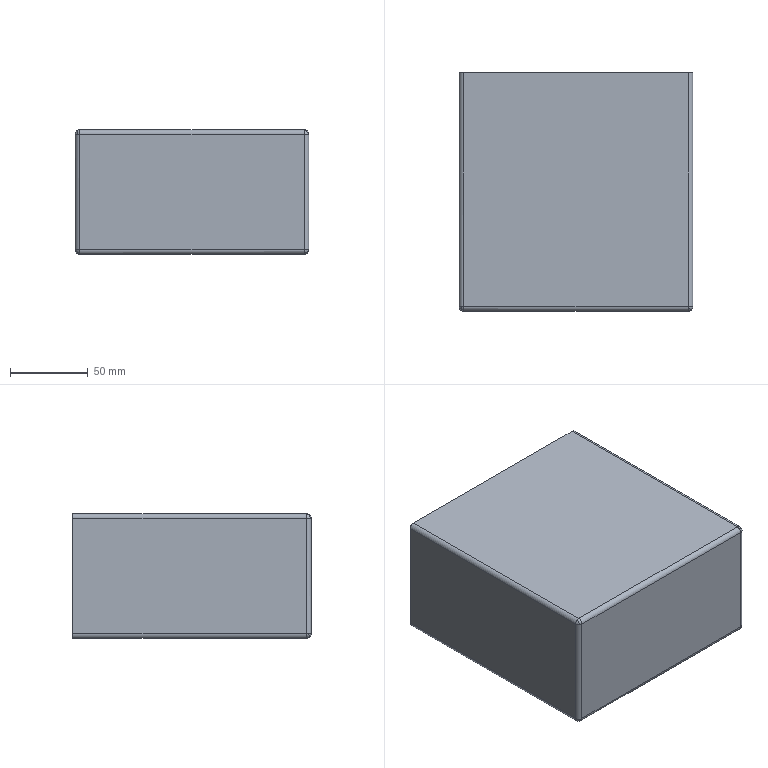Part | SolidWorks | features BaseBody 1 | 1 solid | 43 faces | box 150 x 153 x 80 mm | volume 237530 mm3 | sphere 16 | cylinder 16 | plane 11 | commonest cylinder face diameters 6 x16
STEP:
#1=CARTESIAN_POINT('',(-69.,-147.,-37.));
#2=VERTEX_POINT('',#1);
#3=CARTESIAN_POINT('',(-70.342,-147.,-36.683));
#4=VERTEX_POINT('',#3);
#5=CARTESIAN_POINT('',(-69.,-147.,-34.));
#6=DIRECTION('',(0.,1.,0.));
#7=DIRECTION('',(0.,0.,-1.));
#8=AXIS2_PLACEMENT_3D('',#5,#6,#7);
#9=CIRCLE('',#8,3.);
#10=EDGE_CURVE('',#2,#4,#9,.T.);
#11=ORIENTED_EDGE('',*,*,#10,.T.);
#12=CARTESIAN_POINT('',(-70.342,-149.683,-34.));
#13=VERTEX_POINT('',#12);
#14=CARTESIAN_POINT('',(-69.,-147.,-34.));
#15=DIRECTION('',(-0.8165,0.4082,0.4082));
#16=DIRECTION('',(-0.4472,-0.8944,0.));
#17=AXIS2_PLACEMENT_3D('',#14,#15,#16);
#18=CIRCLE('',#17,3.);
#19=EDGE_CURVE('',#4,#13,#18,.T.);
#20=ORIENTED_EDGE('',*,*,#19,.T.);
#21=CARTESIAN_POINT('',(-69.,-150.,-34.));
#22=VERTEX_POINT('',#21);
#23=CARTESIAN_POINT('',(-69.,-147.,-34.));
#24=DIRECTION('',(0.,0.,-1.));
#25=DIRECTION('',(0.,-1.,0.));
#26=AXIS2_PLACEMENT_3D('',#23,#24,#25);
#27=CIRCLE('',#26,3.);
#28=EDGE_CURVE('',#22,#13,#27,.T.);
#29=ORIENTED_EDGE('',*,*,#28,.F.);
#30=CARTESIAN_POINT('',(-69.,-147.,-34.));
#31=DIRECTION('',(-1.,0.,0.));
#32=DIRECTION('',(0.,0.,-1.));
#33=AXIS2_PLACEMENT_3D('',#30,#31,#32);
#34=CIRCLE('',#33,3.);
#35=EDGE_CURVE('',#2,#22,#34,.T.);
#36=ORIENTED_EDGE('',*,*,#35,.F.);
#37=EDGE_LOOP('',(#11,#20,#29,#36));
#38=FACE_OUTER_BOUND('',#37,.T.);
#39=CARTESIAN_POINT('',(-69.,-147.,-34.));
#40=DIRECTION('',(-0.8165,0.4082,0.4082));
#41=DIRECTION('',(0.5774,0.5774,0.5774));
#42=AXIS2_PLACEMENT_3D('',#39,#40,#41);
#43=SPHERICAL_SURFACE('',#42,3.);
#44=ADVANCED_FACE('',(#38),#43,.F.);
#45=CARTESIAN_POINT('',(-69.,-149.683,35.342));
#46=VERTEX_POINT('',#45);
#47=CARTESIAN_POINT('',(-69.,-147.,37.));
#48=VERTEX_POINT('',#47);
#49=CARTESIAN_POINT('',(-69.,-147.,34.));
#50=DIRECTION('',(-1.,0.,0.));
#51=DIRECTION('',(0.,-1.,0.));
#52=AXIS2_PLACEMENT_3D('',#49,#50,#51);
#53=CIRCLE('',#52,3.);
#54=EDGE_CURVE('',#46,#48,#53,.T.);
#55=ORIENTED_EDGE('',*,*,#54,.F.);
#56=CARTESIAN_POINT('',(-71.683,-147.,35.342));
#57=VERTEX_POINT('',#56);
#58=CARTESIAN_POINT('',(-69.,-147.,34.));
#59=DIRECTION('',(-0.4082,-0.4082,-0.8165));
#60=DIRECTION('',(-0.8944,0.,0.4472));
#61=AXIS2_PLACEMENT_3D('',#58,#59,#60);
#62=CIRCLE('',#61,3.);
#63=EDGE_CURVE('',#46,#57,#62,.T.);
#64=ORIENTED_EDGE('',*,*,#63,.T.);
#65=CARTESIAN_POINT('',(-69.,-147.,34.));
#66=DIRECTION('',(0.,1.,0.));
#67=DIRECTION('',(-1.,0.,0.));
#68=AXIS2_PLACEMENT_3D('',#65,#66,#67);
#69=CIRCLE('',#68,3.);
#70=EDGE_CURVE('',#57,#48,#69,.T.);
#71=ORIENTED_EDGE('',*,*,#70,.T.);
#72=EDGE_LOOP('',(#55,#64,#71));
#73=FACE_OUTER_BOUND('',#72,.T.);
#74=CARTESIAN_POINT('',(-69.,-147.,34.));
#75=DIRECTION('',(-0.4082,-0.4082,-0.8165));
#76=DIRECTION('',(0.5774,0.5774,-0.5774));
#77=AXIS2_PLACEMENT_3D('',#74,#75,#76);
#78=SPHERICAL_SURFACE('',#77,3.);
#79=ADVANCED_FACE('',(#73),#78,.F.);
#80=CARTESIAN_POINT('',(70.342,-149.683,34.));
#81=VERTEX_POINT('',#80);
#82=CARTESIAN_POINT('',(72.,-147.,34.));
#83=VERTEX_POINT('',#82);
#84=CARTESIAN_POINT('',(69.,-147.,34.));
#85=DIRECTION('',(0.,0.,1.));
#86=DIRECTION('',(0.,-1.,0.));
#87=AXIS2_PLACEMENT_3D('',#84,#85,#86);
#88=CIRCLE('',#87,3.);
#89=EDGE_CURVE('',#81,#83,#88,.T.);
#90=ORIENTED_EDGE('',*,*,#89,.F.);
#91=CARTESIAN_POINT('',(70.342,-147.,36.683));
#92=VERTEX_POINT('',#91);
#93=CARTESIAN_POINT('',(69.,-147.,34.));
#94=DIRECTION('',(-0.8165,-0.4082,0.4082));
#95=DIRECTION('',(0.4472,-0.8944,0.));
#96=AXIS2_PLACEMENT_3D('',#93,#94,#95);
#97=CIRCLE('',#96,3.);
#98=EDGE_CURVE('',#81,#92,#97,.T.);
#99=ORIENTED_EDGE('',*,*,#98,.T.);
#100=CARTESIAN_POINT('',(69.,-147.,34.));
#101=DIRECTION('',(0.,1.,0.));
#102=DIRECTION('',(0.,0.,1.));
#103=AXIS2_PLACEMENT_3D('',#100,#101,#102);
#104=CIRCLE('',#103,3.);
#105=EDGE_CURVE('',#92,#83,#104,.T.);
#106=ORIENTED_EDGE('',*,*,#105,.T.);
#107=EDGE_LOOP('',(#90,#99,#106));
#108=FACE_OUTER_BOUND('',#107,.T.);
#109=CARTESIAN_POINT('',(69.,-147.,34.));
#110=DIRECTION('',(-0.8165,-0.4082,0.4082));
#111=DIRECTION('',(-0.5774,0.5774,-0.5774));
#112=AXIS2_PLACEMENT_3D('',#109,#110,#111);
#113=SPHERICAL_SURFACE('',#112,3.);
#114=ADVANCED_FACE('',(#108),#113,.F.);
#115=CARTESIAN_POINT('',(72.,-147.,-34.));
#116=VERTEX_POINT('',#115);
#117=CARTESIAN_POINT('',(71.683,-147.,-35.342));
#118=VERTEX_POINT('',#117);
#119=CARTESIAN_POINT('',(69.,-147.,-34.));
#120=DIRECTION('',(0.,1.,0.));
#121=DIRECTION('',(1.,0.,0.));
#122=AXIS2_PLACEMENT_3D('',#119,#120,#121);
#123=CIRCLE('',#122,3.);
#124=EDGE_CURVE('',#116,#118,#123,.T.);
#125=ORIENTED_EDGE('',*,*,#124,.T.);
#126=CARTESIAN_POINT('',(69.,-149.683,-35.342));
#127=VERTEX_POINT('',#126);
#128=CARTESIAN_POINT('',(69.,-147.,-34.));
#129=DIRECTION('',(-0.4082,0.4082,-0.8165));
#130=DIRECTION('',(-0.8944,0.,0.4472));
#131=AXIS2_PLACEMENT_3D('',#128,#129,#130);
#132=CIRCLE('',#131,3.);
#133=EDGE_CURVE('',#118,#127,#132,.T.);
#134=ORIENTED_EDGE('',*,*,#133,.T.);
#135=CARTESIAN_POINT('',(69.,-150.,-34.));
#136=VERTEX_POINT('',#135);
#137=CARTESIAN_POINT('',(69.,-147.,-34.));
#138=DIRECTION('',(1.,0.,0.));
#139=DIRECTION('',(0.,-1.,0.));
#140=AXIS2_PLACEMENT_3D('',#137,#138,#139);
#141=CIRCLE('',#140,3.);
#142=EDGE_CURVE('',#136,#127,#141,.T.);
#143=ORIENTED_EDGE('',*,*,#142,.F.);
#144=CARTESIAN_POINT('',(69.,-147.,-34.));
#145=DIRECTION('',(0.,0.,-1.));
#146=DIRECTION('',(1.,0.,0.));
#147=AXIS2_PLACEMENT_3D('',#144,#145,#146);
#148=CIRCLE('',#147,3.);
#149=EDGE_CURVE('',#116,#136,#148,.T.);
#150=ORIENTED_EDGE('',*,*,#149,.F.);
#151=EDGE_LOOP('',(#125,#134,#143,#150));
#152=FACE_OUTER_BOUND('',#151,.T.);
#153=CARTESIAN_POINT('',(69.,-147.,-34.));
#154=DIRECTION('',(-0.4082,0.4082,-0.8165));
#155=DIRECTION('',(-0.5774,0.5774,0.5774));
#156=AXIS2_PLACEMENT_3D('',#153,#154,#155);
#157=SPHERICAL_SURFACE('',#156,3.);
#158=ADVANCED_FACE('',(#152),#157,.F.);
#159=CARTESIAN_POINT('',(72.,-153.,-37.));
#160=VERTEX_POINT('',#159);
#161=CARTESIAN_POINT('',(72.,-152.121,-39.121));
#162=VERTEX_POINT('',#161);
#163=CARTESIAN_POINT('',(72.,-150.,-37.));
#164=DIRECTION('',(1.,0.,0.));
#165=DIRECTION('',(0.,-1.,0.));
#166=AXIS2_PLACEMENT_3D('',#163,#164,#165);
#167=CIRCLE('',#166,3.);
#168=EDGE_CURVE('',#160,#162,#167,.T.);
#169=ORIENTED_EDGE('',*,*,#168,.T.);
#170=CARTESIAN_POINT('',(75.,-150.,-37.));
#171=VERTEX_POINT('',#170);
#172=CARTESIAN_POINT('',(72.,-150.,-37.));
#173=DIRECTION('',(0.,-0.7071,0.7071));
#174=DIRECTION('',(0.,-0.7071,-0.7071));
#175=AXIS2_PLACEMENT_3D('',#172,#173,#174);
#176=CIRCLE('',#175,3.);
#177=EDGE_CURVE('',#162,#171,#176,.T.);
#178=ORIENTED_EDGE('',*,*,#177,.T.);
#179=CARTESIAN_POINT('',(72.,-150.,-37.));
#180=DIRECTION('',(0.,0.,-1.));
#181=DIRECTION('',(1.,0.,0.));
#182=AXIS2_PLACEMENT_3D('',#179,#180,#181);
#183=CIRCLE('',#182,3.);
#184=EDGE_CURVE('',#171,#160,#183,.T.);
#185=ORIENTED_EDGE('',*,*,#184,.T.);
#186=EDGE_LOOP('',(#169,#178,#185));
#187=FACE_OUTER_BOUND('',#186,.T.);
#188=CARTESIAN_POINT('',(72.,-150.,-37.));
#189=DIRECTION('',(0.,-0.7071,0.7071));
#190=DIRECTION('',(-0.5774,0.5774,0.5774));
#191=AXIS2_PLACEMENT_3D('',#188,#189,#190);
#192=SPHERICAL_SURFACE('',#191,3.);
#193=ADVANCED_FACE('',(#187),#192,.T.);
#194=CARTESIAN_POINT('',(72.,-150.,40.));
#195=VERTEX_POINT('',#194);
#196=CARTESIAN_POINT('',(72.,-151.342,39.683));
#197=VERTEX_POINT('',#196);
#198=CARTESIAN_POINT('',(72.,-150.,37.));
#199=DIRECTION('',(1.,0.,0.));
#200=DIRECTION('',(0.,0.,1.));
#201=AXIS2_PLACEMENT_3D('',#198,#199,#200);
#202=CIRCLE('',#201,3.);
#203=EDGE_CURVE('',#195,#197,#202,.T.);
#204=ORIENTED_EDGE('',*,*,#203,.T.);
#205=CARTESIAN_POINT('',(74.683,-151.342,37.));
#206=VERTEX_POINT('',#205);
#207=CARTESIAN_POINT('',(72.,-150.,37.));
#208=DIRECTION('',(0.4082,0.8165,0.4082));
#209=DIRECTION('',(0.,-0.4472,0.8944));
#210=AXIS2_PLACEMENT_3D('',#207,#208,#209);
#211=CIRCLE('',#210,3.);
#212=EDGE_CURVE('',#197,#206,#211,.T.);
#213=ORIENTED_EDGE('',*,*,#212,.T.);
#214=CARTESIAN_POINT('',(75.,-150.,37.));
#215=VERTEX_POINT('',#214);
#216=CARTESIAN_POINT('',(72.,-150.,37.));
#217=DIRECTION('',(0.,0.,-1.));
#218=DIRECTION('',(1.,0.,0.));
#219=AXIS2_PLACEMENT_3D('',#216,#217,#218);
#220=CIRCLE('',#219,3.);
#221=EDGE_CURVE('',#215,#206,#220,.T.);
#222=ORIENTED_EDGE('',*,*,#221,.F.);
#223=CARTESIAN_POINT('',(72.,-150.,37.));
#224=DIRECTION('',(0.,1.,0.));
#225=DIRECTION('',(0.,0.,1.));
#226=AXIS2_PLACEMENT_3D('',#223,#224,#225);
#227=CIRCLE('',#226,3.);
#228=EDGE_CURVE('',#195,#215,#227,.T.);
#229=ORIENTED_EDGE('',*,*,#228,.F.);
#230=EDGE_LOOP('',(#204,#213,#222,#229));
#231=FACE_OUTER_BOUND('',#230,.T.);
#232=CARTESIAN_POINT('',(72.,-150.,37.));
#233=DIRECTION('',(0.4082,0.8165,0.4082));
#234=DIRECTION('',(-0.5774,0.5774,-0.5774));
#235=AXIS2_PLACEMENT_3D('',#232,#233,#234);
#236=SPHERICAL_SURFACE('',#235,3.);
#237=ADVANCED_FACE('',(#231),#236,.T.);
#238=CARTESIAN_POINT('',(-72.,-150.,-40.));
#239=VERTEX_POINT('',#238);
#240=CARTESIAN_POINT('',(-72.,-151.342,-39.683));
#241=VERTEX_POINT('',#240);
#242=CARTESIAN_POINT('',(-72.,-150.,-37.));
#243=DIRECTION('',(-1.,0.,0.));
#244=DIRECTION('',(0.,0.,-1.));
#245=AXIS2_PLACEMENT_3D('',#242,#243,#244);
#246=CIRCLE('',#245,3.);
#247=EDGE_CURVE('',#239,#241,#246,.T.);
#248=ORIENTED_EDGE('',*,*,#247,.T.);
#249=CARTESIAN_POINT('',(-74.683,-151.342,-37.));
#250=VERTEX_POINT('',#249);
#251=CARTESIAN_POINT('',(-72.,-150.,-37.));
#252=DIRECTION('',(-0.4082,0.8165,-0.4082));
#253=DIRECTION('',(0.,0.4472,0.8944));
#254=AXIS2_PLACEMENT_3D('',#251,#252,#253);
#255=CIRCLE('',#254,3.);
#256=EDGE_CURVE('',#241,#250,#255,.T.);
#257=ORIENTED_EDGE('',*,*,#256,.T.);
#258=CARTESIAN_POINT('',(-75.,-150.,-37.));
#259=VERTEX_POINT('',#258);
#260=CARTESIAN_POINT('',(-72.,-150.,-37.));
#261=DIRECTION('',(0.,0.,-1.));
#262=DIRECTION('',(0.,-1.,0.));
#263=AXIS2_PLACEMENT_3D('',#260,#261,#262);
#264=CIRCLE('',#263,3.);
#265=EDGE_CURVE('',#250,#259,#264,.T.);
#266=ORIENTED_EDGE('',*,*,#265,.T.);
#267=CARTESIAN_POINT('',(-72.,-150.,-37.));
#268=DIRECTION('',(0.,1.,0.));
#269=DIRECTION('',(0.,0.,-1.));
#270=AXIS2_PLACEMENT_3D('',#267,#268,#269);
#271=CIRCLE('',#270,3.);
#272=EDGE_CURVE('',#239,#259,#271,.T.);
#273=ORIENTED_EDGE('',*,*,#272,.F.);
#274=EDGE_LOOP('',(#248,#257,#266,#273));
#275=FACE_OUTER_BOUND('',#274,.T.);
#276=CARTESIAN_POINT('',(-72.,-150.,-37.));
#277=DIRECTION('',(-0.4082,0.8165,-0.4082));
#278=DIRECTION('',(0.5774,0.5774,0.5774));
#279=AXIS2_PLACEMENT_3D('',#276,#277,#278);
#280=SPHERICAL_SURFACE('',#279,3.);
#281=ADVANCED_FACE('',(#275),#280,.T.);
#282=CARTESIAN_POINT('',(-73.342,-150.,39.683));
#283=VERTEX_POINT('',#282);
#284=CARTESIAN_POINT('',(-72.,-150.,40.));
#285=VERTEX_POINT('',#284);
#286=CARTESIAN_POINT('',(-72.,-150.,37.));
#287=DIRECTION('',(0.,1.,0.));
#288=DIRECTION('',(-1.,0.,0.));
#289=AXIS2_PLACEMENT_3D('',#286,#287,#288);
#290=CIRCLE('',#289,3.);
#291=EDGE_CURVE('',#283,#285,#290,.T.);
#292=ORIENTED_EDGE('',*,*,#291,.F.);
#293=CARTESIAN_POINT('',(-73.342,-152.683,37.));
#294=VERTEX_POINT('',#293);
#295=CARTESIAN_POINT('',(-72.,-150.,37.));
#296=DIRECTION('',(0.8165,-0.4082,0.4082));
#297=DIRECTION('',(0.4472,0.,-0.8944));
#298=AXIS2_PLACEMENT_3D('',#295,#296,#297);
#299=CIRCLE('',#298,3.);
#300=EDGE_CURVE('',#283,#294,#299,.T.);
#301=ORIENTED_EDGE('',*,*,#300,.T.);
#302=CARTESIAN_POINT('',(-72.,-153.,37.));
#303=VERTEX_POINT('',#302);
#304=CARTESIAN_POINT('',(-72.,-150.,37.));
#305=DIRECTION('',(0.,0.,1.));
#306=DIRECTION('',(-1.,0.,0.));
#307=AXIS2_PLACEMENT_3D('',#304,#305,#306);
#308=CIRCLE('',#307,3.);
#309=EDGE_CURVE('',#294,#303,#308,.T.);
#310=ORIENTED_EDGE('',*,*,#309,.T.);
#311=CARTESIAN_POINT('',(-72.,-150.,37.));
#312=DIRECTION('',(1.,0.,0.));
#313=DIRECTION('',(0.,0.,1.));
#314=AXIS2_PLACEMENT_3D('',#311,#312,#313);
#315=CIRCLE('',#314,3.);
#316=EDGE_CURVE('',#285,#303,#315,.T.);
#317=ORIENTED_EDGE('',*,*,#316,.F.);
#318=EDGE_LOOP('',(#292,#301,#310,#317));
#319=FACE_OUTER_BOUND('',#318,.T.);
#320=CARTESIAN_POINT('',(-72.,-150.,37.));
#321=DIRECTION('',(0.8165,-0.4082,0.4082));
#322=DIRECTION('',(0.5774,0.5774,-0.5774));
#323=AXIS2_PLACEMENT_3D('',#320,#321,#322);
#324=SPHERICAL_SURFACE('',#323,3.);
#325=ADVANCED_FACE('',(#319),#324,.T.);
#326=CARTESIAN_POINT('',(72.,-153.,37.));
#327=VERTEX_POINT('',#326);
#328=CARTESIAN_POINT('',(-72.,-153.,37.));
#329=DIRECTION('',(1.,0.,0.));
#330=VECTOR('',#329,1000.);
#331=LINE('',#328,#330);
#332=EDGE_CURVE('',#303,#327,#331,.T.);
#333=ORIENTED_EDGE('',*,*,#332,.F.);
#334=CARTESIAN_POINT('',(-72.,-153.,-37.));
#335=VERTEX_POINT('',#334);
#336=CARTESIAN_POINT('',(-72.,-153.,-37.));
#337=DIRECTION('',(0.,0.,1.));
#338=VECTOR('',#337,1000.);
#339=LINE('',#336,#338);
#340=EDGE_CURVE('',#335,#303,#339,.T.);
#341=ORIENTED_EDGE('',*,*,#340,.F.);
#342=CARTESIAN_POINT('',(72.,-153.,-37.));
#343=DIRECTION('',(-1.,0.,0.));
#344=VECTOR('',#343,1000.);
#345=LINE('',#342,#344);
#346=EDGE_CURVE('',#160,#335,#345,.T.);
#347=ORIENTED_EDGE('',*,*,#346,.F.);
#348=CARTESIAN_POINT('',(72.,-153.,37.));
#349=DIRECTION('',(0.,0.,-1.));
#350=VECTOR('',#349,1000.);
#351=LINE('',#348,#350);
#352=EDGE_CURVE('',#327,#160,#351,.T.);
#353=ORIENTED_EDGE('',*,*,#352,.F.);
#354=EDGE_LOOP('',(#333,#341,#347,#353));
#355=FACE_OUTER_BOUND('',#354,.T.);
#356=CARTESIAN_POINT('',(0.,-153.,0.));
#357=DIRECTION('',(0.,-1.,0.));
#358=DIRECTION('',(0.,0.,-1.));
#359=AXIS2_PLACEMENT_3D('',#356,#357,#358);
#360=PLANE('',#359);
#361=ADVANCED_FACE('',(#355),#360,.T.);
#362=CARTESIAN_POINT('',(-72.,-150.,-37.));
#363=DIRECTION('',(0.,0.,-1.));
#364=DIRECTION('',(0.,-1.,0.));
#365=AXIS2_PLACEMENT_3D('',#362,#363,#364);
#366=CIRCLE('',#365,3.);
#367=EDGE_CURVE('',#335,#250,#366,.T.);
#368=ORIENTED_EDGE('',*,*,#367,.F.);
#369=ORIENTED_EDGE('',*,*,#340,.T.);
#370=ORIENTED_EDGE('',*,*,#309,.F.);
#371=CARTESIAN_POINT('',(-75.,-150.,37.));
#372=VERTEX_POINT('',#371);
#373=CARTESIAN_POINT('',(-72.,-150.,37.));
#374=DIRECTION('',(0.,0.,1.));
#375=DIRECTION('',(-1.,0.,0.));
#376=AXIS2_PLACEMENT_3D('',#373,#374,#375);
#377=CIRCLE('',#376,3.);
#378=EDGE_CURVE('',#372,#294,#377,.T.);
#379=ORIENTED_EDGE('',*,*,#378,.F.);
#380=CARTESIAN_POINT('',(-75.,-150.,-37.));
#381=DIRECTION('',(0.,0.,1.));
#382=VECTOR('',#381,1000.);
#383=LINE('',#380,#382);
#384=EDGE_CURVE('',#259,#372,#383,.T.);
#385=ORIENTED_EDGE('',*,*,#384,.F.);
#386=ORIENTED_EDGE('',*,*,#265,.F.);
#387=EDGE_LOOP('',(#368,#369,#370,#379,#385,#386));
#388=FACE_OUTER_BOUND('',#387,.T.);
#389=CARTESIAN_POINT('',(-72.,-150.,37.));
#390=DIRECTION('',(0.,0.,-1.));
#391=DIRECTION('',(-1.,0.,0.));
#392=AXIS2_PLACEMENT_3D('',#389,#390,#391);
#393=CYLINDRICAL_SURFACE('',#392,3.);
#394=ADVANCED_FACE('',(#388),#393,.T.);
#395=ORIENTED_EDGE('',*,*,#168,.F.);
#396=ORIENTED_EDGE('',*,*,#346,.T.);
#397=CARTESIAN_POINT('',(-72.,-150.,-37.));
#398=DIRECTION('',(-1.,0.,0.));
#399=DIRECTION('',(0.,0.,-1.));
#400=AXIS2_PLACEMENT_3D('',#397,#398,#399);
#401=CIRCLE('',#400,3.);
#402=EDGE_CURVE('',#241,#335,#401,.T.);
#403=ORIENTED_EDGE('',*,*,#402,.F.);
#404=ORIENTED_EDGE('',*,*,#247,.F.);
#405=CARTESIAN_POINT('',(72.,-150.,-40.));
#406=VERTEX_POINT('',#405);
#407=CARTESIAN_POINT('',(72.,-150.,-40.));
#408=DIRECTION('',(-1.,0.,0.));
#409=VECTOR('',#408,1000.);
#410=LINE('',#407,#409);
#411=EDGE_CURVE('',#406,#239,#410,.T.);
#412=ORIENTED_EDGE('',*,*,#411,.F.);
#413=CARTESIAN_POINT('',(72.,-150.,-37.));
#414=DIRECTION('',(1.,0.,0.));
#415=DIRECTION('',(0.,-1.,0.));
#416=AXIS2_PLACEMENT_3D('',#413,#414,#415);
#417=CIRCLE('',#416,3.);
#418=EDGE_CURVE('',#162,#406,#417,.T.);
#419=ORIENTED_EDGE('',*,*,#418,.F.);
#420=EDGE_LOOP('',(#395,#396,#403,#404,#412,#419));
#421=FACE_OUTER_BOUND('',#420,.T.);
#422=CARTESIAN_POINT('',(-72.,-150.,-37.));
#423=DIRECTION('',(1.,0.,0.));
#424=DIRECTION('',(0.,0.,-1.));
#425=AXIS2_PLACEMENT_3D('',#422,#423,#424);
#426=CYLINDRICAL_SURFACE('',#425,3.);
#427=ADVANCED_FACE('',(#421),#426,.T.);
#428=ORIENTED_EDGE('',*,*,#300,.F.);
#429=CARTESIAN_POINT('',(-72.,-150.,37.));
#430=DIRECTION('',(0.,1.,0.));
#431=DIRECTION('',(-1.,0.,0.));
#432=AXIS2_PLACEMENT_3D('',#429,#430,#431);
#433=CIRCLE('',#432,3.);
#434=EDGE_CURVE('',#372,#283,#433,.T.);
#435=ORIENTED_EDGE('',*,*,#434,.F.);
#436=ORIENTED_EDGE('',*,*,#378,.T.);
#437=EDGE_LOOP('',(#428,#435,#436));
#438=FACE_OUTER_BOUND('',#437,.T.);
#439=CARTESIAN_POINT('',(-72.,-150.,37.));
#440=DIRECTION('',(0.8165,-0.4082,0.4082));
#441=DIRECTION('',(0.5774,0.5774,-0.5774));
#442=AXIS2_PLACEMENT_3D('',#439,#440,#441);
#443=SPHERICAL_SURFACE('',#442,3.);
#444=ADVANCED_FACE('',(#438),#443,.T.);
#445=CARTESIAN_POINT('',(-75.,0.,37.));
#446=VERTEX_POINT('',#445);
#447=CARTESIAN_POINT('',(-72.,0.,40.));
#448=VERTEX_POINT('',#447);
#449=CARTESIAN_POINT('',(-72.,0.,37.));
#450=DIRECTION('',(0.,1.,0.));
#451=DIRECTION('',(-1.,0.,0.));
#452=AXIS2_PLACEMENT_3D('',#449,#450,#451);
#453=CIRCLE('',#452,3.);
#454=EDGE_CURVE('',#446,#448,#453,.T.);
#455=ORIENTED_EDGE('',*,*,#454,.F.);
#456=CARTESIAN_POINT('',(-75.,-150.,37.));
#457=DIRECTION('',(0.,1.,0.));
#458=VECTOR('',#457,1000.);
#459=LINE('',#456,#458);
#460=EDGE_CURVE('',#372,#446,#459,.T.);
#461=ORIENTED_EDGE('',*,*,#460,.F.);
#462=ORIENTED_EDGE('',*,*,#434,.T.);
#463=ORIENTED_EDGE('',*,*,#291,.T.);
#464=CARTESIAN_POINT('',(-72.,0.,40.));
#465=DIRECTION('',(0.,-1.,0.));
#466=VECTOR('',#465,1000.);
#467=LINE('',#464,#466);
#468=EDGE_CURVE('',#448,#285,#467,.T.);
#469=ORIENTED_EDGE('',*,*,#468,.F.);
#470=EDGE_LOOP('',(#455,#461,#462,#463,#469));
#471=FACE_OUTER_BOUND('',#470,.T.);
#472=CARTESIAN_POINT('',(-72.,0.,37.));
#473=DIRECTION('',(0.,-1.,0.));
#474=DIRECTION('',(-1.,0.,0.));
#475=AXIS2_PLACEMENT_3D('',#472,#473,#474);
#476=CYLINDRICAL_SURFACE('',#475,3.);
#477=ADVANCED_FACE('',(#471),#476,.T.);
#478=CARTESIAN_POINT('',(-75.,0.,-37.));
#479=VERTEX_POINT('',#478);
#480=CARTESIAN_POINT('',(-75.,-150.,-37.));
#481=DIRECTION('',(0.,1.,0.));
#482=VECTOR('',#481,1000.);
#483=LINE('',#480,#482);
#484=EDGE_CURVE('',#259,#479,#483,.T.);
#485=ORIENTED_EDGE('',*,*,#484,.F.);
#486=ORIENTED_EDGE('',*,*,#384,.T.);
#487=ORIENTED_EDGE('',*,*,#460,.T.);
#488=CARTESIAN_POINT('',(-75.,0.,-37.));
#489=DIRECTION('',(0.,0.,1.));
#490=VECTOR('',#489,1000.);
#491=LINE('',#488,#490);
#492=EDGE_CURVE('',#479,#446,#491,.T.);
#493=ORIENTED_EDGE('',*,*,#492,.F.);
#494=EDGE_LOOP('',(#485,#486,#487,#493));
#495=FACE_OUTER_BOUND('',#494,.T.);
#496=CARTESIAN_POINT('',(-75.,0.,40.));
#497=DIRECTION('',(-1.,0.,0.));
#498=DIRECTION('',(0.,0.,1.));
#499=AXIS2_PLACEMENT_3D('',#496,#497,#498);
#500=PLANE('',#499);
#501=ADVANCED_FACE('',(#495),#500,.T.);
#502=CARTESIAN_POINT('',(72.,0.,-40.));
#503=VERTEX_POINT('',#502);
#504=CARTESIAN_POINT('',(72.,-150.,-40.));
#505=DIRECTION('',(0.,1.,0.));
#506=VECTOR('',#505,1000.);
#507=LINE('',#504,#506);
#508=EDGE_CURVE('',#406,#503,#507,.T.);
#509=ORIENTED_EDGE('',*,*,#508,.F.);
#510=ORIENTED_EDGE('',*,*,#411,.T.);
#511=CARTESIAN_POINT('',(-72.,0.,-40.));
#512=VERTEX_POINT('',#511);
#513=CARTESIAN_POINT('',(-72.,0.,-40.));
#514=DIRECTION('',(0.,-1.,0.));
#515=VECTOR('',#514,1000.);
#516=LINE('',#513,#515);
#517=EDGE_CURVE('',#512,#239,#516,.T.);
#518=ORIENTED_EDGE('',*,*,#517,.F.);
#519=CARTESIAN_POINT('',(72.,0.,-40.));
#520=DIRECTION('',(-1.,0.,0.));
#521=VECTOR('',#520,1000.);
#522=LINE('',#519,#521);
#523=EDGE_CURVE('',#503,#512,#522,.T.);
#524=ORIENTED_EDGE('',*,*,#523,.F.);
#525=EDGE_LOOP('',(#509,#510,#518,#524));
#526=FACE_OUTER_BOUND('',#525,.T.);
#527=CARTESIAN_POINT('',(-75.,0.,-40.));
#528=DIRECTION('',(0.,0.,-1.));
#529=DIRECTION('',(0.,-1.,0.));
#530=AXIS2_PLACEMENT_3D('',#527,#528,#529);
#531=PLANE('',#530);
#532=ADVANCED_FACE('',(#526),#531,.T.);
#533=ORIENTED_EDGE('',*,*,#256,.F.);
#534=ORIENTED_EDGE('',*,*,#402,.T.);
#535=ORIENTED_EDGE('',*,*,#367,.T.);
#536=EDGE_LOOP('',(#533,#534,#535));
#537=FACE_OUTER_BOUND('',#536,.T.);
#538=CARTESIAN_POINT('',(-72.,-150.,-37.));
#539=DIRECTION('',(-0.4082,0.8165,-0.4082));
#540=DIRECTION('',(0.5774,0.5774,0.5774));
#541=AXIS2_PLACEMENT_3D('',#538,#539,#540);
#542=SPHERICAL_SURFACE('',#541,3.);
#543=ADVANCED_FACE('',(#537),#542,.T.);
#544=CARTESIAN_POINT('',(-72.,0.,-37.));
#545=DIRECTION('',(0.,1.,0.));
#546=DIRECTION('',(0.,0.,-1.));
#547=AXIS2_PLACEMENT_3D('',#544,#545,#546);
#548=CIRCLE('',#547,3.);
#549=EDGE_CURVE('',#512,#479,#548,.T.);
#550=ORIENTED_EDGE('',*,*,#549,.F.);
#551=ORIENTED_EDGE('',*,*,#517,.T.);
#552=ORIENTED_EDGE('',*,*,#272,.T.);
#553=ORIENTED_EDGE('',*,*,#484,.T.);
#554=EDGE_LOOP('',(#550,#551,#552,#553));
#555=FACE_OUTER_BOUND('',#554,.T.);
#556=CARTESIAN_POINT('',(-72.,0.,-37.));
#557=DIRECTION('',(0.,-1.,0.));
#558=DIRECTION('',(0.,0.,-1.));
#559=AXIS2_PLACEMENT_3D('',#556,#557,#558);
#560=CYLINDRICAL_SURFACE('',#559,3.);
#561=ADVANCED_FACE('',(#555),#560,.T.);
#562=CARTESIAN_POINT('',(-72.,-147.,34.));
#563=VERTEX_POINT('',#562);
#564=CARTESIAN_POINT('',(-69.,-147.,34.));
#565=DIRECTION('',(0.,1.,0.));
#566=DIRECTION('',(-1.,0.,0.));
#567=AXIS2_PLACEMENT_3D('',#564,#565,#566);
#568=CIRCLE('',#567,3.);
#569=EDGE_CURVE('',#563,#57,#568,.T.);
#570=ORIENTED_EDGE('',*,*,#569,.F.);
#571=CARTESIAN_POINT('',(-72.,0.,34.));
#572=VERTEX_POINT('',#571);
#573=CARTESIAN_POINT('',(-72.,0.,34.));
#574=DIRECTION('',(0.,-1.,0.));
#575=VECTOR('',#574,1000.);
#576=LINE('',#573,#575);
#577=EDGE_CURVE('',#572,#563,#576,.T.);
#578=ORIENTED_EDGE('',*,*,#577,.F.);
#579=CARTESIAN_POINT('',(-69.,0.,37.));
#580=VERTEX_POINT('',#579);
#581=CARTESIAN_POINT('',(-69.,0.,34.));
#582=DIRECTION('',(0.,-1.,0.));
#583=DIRECTION('',(0.,0.,1.));
#584=AXIS2_PLACEMENT_3D('',#581,#582,#583);
#585=CIRCLE('',#584,3.);
#586=EDGE_CURVE('',#580,#572,#585,.T.);
#587=ORIENTED_EDGE('',*,*,#586,.F.);
#588=CARTESIAN_POINT('',(-69.,-147.,37.));
#589=DIRECTION('',(0.,1.,0.));
#590=VECTOR('',#589,1000.);
#591=LINE('',#588,#590);
#592=EDGE_CURVE('',#48,#580,#591,.T.);
#593=ORIENTED_EDGE('',*,*,#592,.F.);
#594=ORIENTED_EDGE('',*,*,#70,.F.);
#595=EDGE_LOOP('',(#570,#578,#587,#593,#594));
#596=FACE_OUTER_BOUND('',#595,.T.);
#597=CARTESIAN_POINT('',(-69.,0.,34.));
#598=DIRECTION('',(0.,-1.,0.));
#599=DIRECTION('',(0.,0.,1.));
#600=AXIS2_PLACEMENT_3D('',#597,#598,#599);
#601=CYLINDRICAL_SURFACE('',#600,3.);
#602=ADVANCED_FACE('',(#596),#601,.F.);
#603=CARTESIAN_POINT('',(72.,0.,40.));
#604=VERTEX_POINT('',#603);
#605=CARTESIAN_POINT('',(72.,0.,40.));
#606=DIRECTION('',(0.,-1.,0.));
#607=VECTOR('',#606,1000.);
#608=LINE('',#605,#607);
#609=EDGE_CURVE('',#604,#195,#608,.T.);
#610=ORIENTED_EDGE('',*,*,#609,.F.);
#611=CARTESIAN_POINT('',(-72.,0.,40.));
#612=DIRECTION('',(1.,0.,0.));
#613=VECTOR('',#612,1000.);
#614=LINE('',#611,#613);
#615=EDGE_CURVE('',#448,#604,#614,.T.);
#616=ORIENTED_EDGE('',*,*,#615,.F.);
#617=ORIENTED_EDGE('',*,*,#468,.T.);
#618=CARTESIAN_POINT('',(72.,-150.,40.));
#619=DIRECTION('',(-1.,0.,0.));
#620=VECTOR('',#619,1000.);
#621=LINE('',#618,#620);
#622=EDGE_CURVE('',#195,#285,#621,.T.);
#623=ORIENTED_EDGE('',*,*,#622,.F.);
#624=EDGE_LOOP('',(#610,#616,#617,#623));
#625=FACE_OUTER_BOUND('',#624,.T.);
#626=CARTESIAN_POINT('',(75.,0.,40.));
#627=DIRECTION('',(0.,0.,1.));
#628=DIRECTION('',(1.,0.,0.));
#629=AXIS2_PLACEMENT_3D('',#626,#627,#628);
#630=PLANE('',#629);
#631=ADVANCED_FACE('',(#625),#630,.T.);
#632=ORIENTED_EDGE('',*,*,#203,.F.);
#633=ORIENTED_EDGE('',*,*,#622,.T.);
#634=ORIENTED_EDGE('',*,*,#316,.T.);
#635=ORIENTED_EDGE('',*,*,#332,.T.);
#636=CARTESIAN_POINT('',(72.,-150.,37.));
#637=DIRECTION('',(1.,0.,0.));
#638=DIRECTION('',(0.,0.,1.));
#639=AXIS2_PLACEMENT_3D('',#636,#637,#638);
#640=CIRCLE('',#639,3.);
#641=EDGE_CURVE('',#197,#327,#640,.T.);
#642=ORIENTED_EDGE('',*,*,#641,.F.);
#643=EDGE_LOOP('',(#632,#633,#634,#635,#642));
#644=FACE_OUTER_BOUND('',#643,.T.);
#645=CARTESIAN_POINT('',(72.,-150.,37.));
#646=DIRECTION('',(-1.,0.,0.));
#647=DIRECTION('',(0.,0.,1.));
#648=AXIS2_PLACEMENT_3D('',#645,#646,#647);
#649=CYLINDRICAL_SURFACE('',#648,3.);
#650=ADVANCED_FACE('',(#644),#649,.T.);
#651=ORIENTED_EDGE('',*,*,#212,.F.);
#652=ORIENTED_EDGE('',*,*,#641,.T.);
#653=CARTESIAN_POINT('',(72.,-150.,37.));
#654=DIRECTION('',(0.,0.,-1.));
#655=DIRECTION('',(1.,0.,0.));
#656=AXIS2_PLACEMENT_3D('',#653,#654,#655);
#657=CIRCLE('',#656,3.);
#658=EDGE_CURVE('',#206,#327,#657,.T.);
#659=ORIENTED_EDGE('',*,*,#658,.F.);
#660=EDGE_LOOP('',(#651,#652,#659));
#661=FACE_OUTER_BOUND('',#660,.T.);
#662=CARTESIAN_POINT('',(72.,-150.,37.));
#663=DIRECTION('',(0.4082,0.8165,0.4082));
#664=DIRECTION('',(-0.5774,0.5774,-0.5774));
#665=AXIS2_PLACEMENT_3D('',#662,#663,#664);
#666=SPHERICAL_SURFACE('',#665,3.);
#667=ADVANCED_FACE('',(#661),#666,.T.);
#668=CARTESIAN_POINT('',(75.,0.,37.));
#669=VERTEX_POINT('',#668);
#670=CARTESIAN_POINT('',(72.,0.,37.));
#671=DIRECTION('',(0.,1.,0.));
#672=DIRECTION('',(0.,0.,1.));
#673=AXIS2_PLACEMENT_3D('',#670,#671,#672);
#674=CIRCLE('',#673,3.);
#675=EDGE_CURVE('',#604,#669,#674,.T.);
#676=ORIENTED_EDGE('',*,*,#675,.F.);
#677=ORIENTED_EDGE('',*,*,#609,.T.);
#678=ORIENTED_EDGE('',*,*,#228,.T.);
#679=CARTESIAN_POINT('',(75.,0.,37.));
#680=DIRECTION('',(0.,-1.,0.));
#681=VECTOR('',#680,1000.);
#682=LINE('',#679,#681);
#683=EDGE_CURVE('',#669,#215,#682,.T.);
#684=ORIENTED_EDGE('',*,*,#683,.F.);
#685=EDGE_LOOP('',(#676,#677,#678,#684));
#686=FACE_OUTER_BOUND('',#685,.T.);
#687=CARTESIAN_POINT('',(72.,0.,37.));
#688=DIRECTION('',(0.,-1.,0.));
#689=DIRECTION('',(0.,0.,1.));
#690=AXIS2_PLACEMENT_3D('',#687,#688,#689);
#691=CYLINDRICAL_SURFACE('',#690,3.);
#692=ADVANCED_FACE('',(#686),#691,.T.);
#693=CARTESIAN_POINT('',(69.,-147.,37.));
#694=VERTEX_POINT('',#693);
#695=CARTESIAN_POINT('',(-69.,-147.,37.));
#696=DIRECTION('',(1.,0.,0.));
#697=VECTOR('',#696,1000.);
#698=LINE('',#695,#697);
#699=EDGE_CURVE('',#48,#694,#698,.T.);
#700=ORIENTED_EDGE('',*,*,#699,.F.);
#701=ORIENTED_EDGE('',*,*,#592,.T.);
#702=CARTESIAN_POINT('',(69.,0.,37.));
#703=VERTEX_POINT('',#702);
#704=CARTESIAN_POINT('',(69.,0.,37.));
#705=DIRECTION('',(-1.,0.,0.));
#706=VECTOR('',#705,1000.);
#707=LINE('',#704,#706);
#708=EDGE_CURVE('',#703,#580,#707,.T.);
#709=ORIENTED_EDGE('',*,*,#708,.F.);
#710=CARTESIAN_POINT('',(69.,-147.,37.));
#711=DIRECTION('',(0.,1.,0.));
#712=VECTOR('',#711,1000.);
#713=LINE('',#710,#712);
#714=EDGE_CURVE('',#694,#703,#713,.T.);
#715=ORIENTED_EDGE('',*,*,#714,.F.);
#716=EDGE_LOOP('',(#700,#701,#709,#715));
#717=FACE_OUTER_BOUND('',#716,.T.);
#718=CARTESIAN_POINT('',(-72.,0.,37.));
#719=DIRECTION('',(0.,0.,-1.));
#720=DIRECTION('',(0.,-1.,0.));
#721=AXIS2_PLACEMENT_3D('',#718,#719,#720);
#722=PLANE('',#721);
#723=ADVANCED_FACE('',(#717),#722,.T.);
#724=CARTESIAN_POINT('',(69.,-147.,34.));
#725=DIRECTION('',(0.,1.,0.));
#726=DIRECTION('',(0.,0.,1.));
#727=AXIS2_PLACEMENT_3D('',#724,#725,#726);
#728=CIRCLE('',#727,3.);
#729=EDGE_CURVE('',#694,#92,#728,.T.);
#730=ORIENTED_EDGE('',*,*,#729,.F.);
#731=ORIENTED_EDGE('',*,*,#714,.T.);
#732=CARTESIAN_POINT('',(72.,0.,34.));
#733=VERTEX_POINT('',#732);
#734=CARTESIAN_POINT('',(69.,0.,34.));
#735=DIRECTION('',(0.,-1.,0.));
#736=DIRECTION('',(1.,0.,0.));
#737=AXIS2_PLACEMENT_3D('',#734,#735,#736);
#738=CIRCLE('',#737,3.);
#739=EDGE_CURVE('',#733,#703,#738,.T.);
#740=ORIENTED_EDGE('',*,*,#739,.F.);
#741=CARTESIAN_POINT('',(72.,-147.,34.));
#742=DIRECTION('',(0.,1.,0.));
#743=VECTOR('',#742,1000.);
#744=LINE('',#741,#743);
#745=EDGE_CURVE('',#83,#733,#744,.T.);
#746=ORIENTED_EDGE('',*,*,#745,.F.);
#747=ORIENTED_EDGE('',*,*,#105,.F.);
#748=EDGE_LOOP('',(#730,#731,#740,#746,#747));
#749=FACE_OUTER_BOUND('',#748,.T.);
#750=CARTESIAN_POINT('',(69.,0.,34.));
#751=DIRECTION('',(0.,-1.,0.));
#752=DIRECTION('',(1.,0.,0.));
#753=AXIS2_PLACEMENT_3D('',#750,#751,#752);
#754=CYLINDRICAL_SURFACE('',#753,3.);
#755=ADVANCED_FACE('',(#749),#754,.F.);
#756=CARTESIAN_POINT('',(72.,0.,-34.));
#757=VERTEX_POINT('',#756);
#758=CARTESIAN_POINT('',(72.,0.,34.));
#759=DIRECTION('',(0.,0.,-1.));
#760=VECTOR('',#759,1000.);
#761=LINE('',#758,#760);
#762=EDGE_CURVE('',#733,#757,#761,.T.);
#763=ORIENTED_EDGE('',*,*,#762,.F.);
#764=ORIENTED_EDGE('',*,*,#739,.T.);
#765=ORIENTED_EDGE('',*,*,#708,.T.);
#766=ORIENTED_EDGE('',*,*,#586,.T.);
#767=CARTESIAN_POINT('',(-72.,0.,-34.));
#768=VERTEX_POINT('',#767);
#769=CARTESIAN_POINT('',(-72.,0.,-34.));
#770=DIRECTION('',(0.,0.,1.));
#771=VECTOR('',#770,1000.);
#772=LINE('',#769,#771);
#773=EDGE_CURVE('',#768,#572,#772,.T.);
#774=ORIENTED_EDGE('',*,*,#773,.F.);
#775=CARTESIAN_POINT('',(-69.,0.,-37.));
#776=VERTEX_POINT('',#775);
#777=CARTESIAN_POINT('',(-69.,0.,-34.));
#778=DIRECTION('',(0.,1.,0.));
#779=DIRECTION('',(0.,0.,-1.));
#780=AXIS2_PLACEMENT_3D('',#777,#778,#779);
#781=CIRCLE('',#780,3.);
#782=EDGE_CURVE('',#776,#768,#781,.T.);
#783=ORIENTED_EDGE('',*,*,#782,.F.);
#784=CARTESIAN_POINT('',(69.,0.,-37.));
#785=VERTEX_POINT('',#784);
#786=CARTESIAN_POINT('',(69.,0.,-37.));
#787=DIRECTION('',(-1.,0.,0.));
#788=VECTOR('',#787,1000.);
#789=LINE('',#786,#788);
#790=EDGE_CURVE('',#785,#776,#789,.T.);
#791=ORIENTED_EDGE('',*,*,#790,.F.);
#792=CARTESIAN_POINT('',(69.,0.,-34.));
#793=DIRECTION('',(0.,1.,0.));
#794=DIRECTION('',(1.,0.,0.));
#795=AXIS2_PLACEMENT_3D('',#792,#793,#794);
#796=CIRCLE('',#795,3.);
#797=EDGE_CURVE('',#757,#785,#796,.T.);
#798=ORIENTED_EDGE('',*,*,#797,.F.);
#799=EDGE_LOOP('',(#763,#764,#765,#766,#774,#783,#791,#798));
#800=FACE_BOUND('',#799,.T.);
#801=CARTESIAN_POINT('',(75.,0.,-37.));
#802=VERTEX_POINT('',#801);
#803=CARTESIAN_POINT('',(72.,0.,-37.));
#804=DIRECTION('',(0.,-1.,0.));
#805=DIRECTION('',(0.,0.,-1.));
#806=AXIS2_PLACEMENT_3D('',#803,#804,#805);
#807=CIRCLE('',#806,3.);
#808=EDGE_CURVE('',#503,#802,#807,.T.);
#809=ORIENTED_EDGE('',*,*,#808,.F.);
#810=ORIENTED_EDGE('',*,*,#523,.T.);
#811=ORIENTED_EDGE('',*,*,#549,.T.);
#812=ORIENTED_EDGE('',*,*,#492,.T.);
#813=ORIENTED_EDGE('',*,*,#454,.T.);
#814=ORIENTED_EDGE('',*,*,#615,.T.);
#815=ORIENTED_EDGE('',*,*,#675,.T.);
#816=CARTESIAN_POINT('',(75.,0.,-37.));
#817=DIRECTION('',(0.,0.,1.));
#818=VECTOR('',#817,1000.);
#819=LINE('',#816,#818);
#820=EDGE_CURVE('',#802,#669,#819,.T.);
#821=ORIENTED_EDGE('',*,*,#820,.F.);
#822=EDGE_LOOP('',(#809,#810,#811,#812,#813,#814,#815,#821));
#823=FACE_OUTER_BOUND('',#822,.T.);
#824=CARTESIAN_POINT('',(0.,0.,0.));
#825=DIRECTION('',(0.,1.,0.));
#826=DIRECTION('',(1.,0.,0.));
#827=AXIS2_PLACEMENT_3D('',#824,#825,#826);
#828=PLANE('',#827);
#829=ADVANCED_FACE('',(#800,#823),#828,.T.);
#830=CARTESIAN_POINT('',(75.,0.,-37.));
#831=DIRECTION('',(0.,-1.,0.));
#832=VECTOR('',#831,1000.);
#833=LINE('',#830,#832);
#834=EDGE_CURVE('',#802,#171,#833,.T.);
#835=ORIENTED_EDGE('',*,*,#834,.F.);
#836=ORIENTED_EDGE('',*,*,#820,.T.);
#837=ORIENTED_EDGE('',*,*,#683,.T.);
#838=CARTESIAN_POINT('',(75.,-150.,-37.));
#839=DIRECTION('',(0.,0.,1.));
#840=VECTOR('',#839,1000.);
#841=LINE('',#838,#840);
#842=EDGE_CURVE('',#171,#215,#841,.T.);
#843=ORIENTED_EDGE('',*,*,#842,.F.);
#844=EDGE_LOOP('',(#835,#836,#837,#843));
#845=FACE_OUTER_BOUND('',#844,.T.);
#846=CARTESIAN_POINT('',(75.,0.,-40.));
#847=DIRECTION('',(1.,0.,0.));
#848=DIRECTION('',(0.,1.,0.));
#849=AXIS2_PLACEMENT_3D('',#846,#847,#848);
#850=PLANE('',#849);
#851=ADVANCED_FACE('',(#845),#850,.T.);
#852=ORIENTED_EDGE('',*,*,#184,.F.);
#853=ORIENTED_EDGE('',*,*,#842,.T.);
#854=ORIENTED_EDGE('',*,*,#221,.T.);
#855=ORIENTED_EDGE('',*,*,#658,.T.);
#856=ORIENTED_EDGE('',*,*,#352,.T.);
#857=EDGE_LOOP('',(#852,#853,#854,#855,#856));
#858=FACE_OUTER_BOUND('',#857,.T.);
#859=CARTESIAN_POINT('',(72.,-150.,-37.));
#860=DIRECTION('',(0.,0.,1.));
#861=DIRECTION('',(1.,0.,0.));
#862=AXIS2_PLACEMENT_3D('',#859,#860,#861);
#863=CYLINDRICAL_SURFACE('',#862,3.);
#864=ADVANCED_FACE('',(#858),#863,.T.);
#865=ORIENTED_EDGE('',*,*,#177,.F.);
#866=ORIENTED_EDGE('',*,*,#418,.T.);
#867=CARTESIAN_POINT('',(72.,-150.,-37.));
#868=DIRECTION('',(0.,1.,0.));
#869=DIRECTION('',(1.,0.,0.));
#870=AXIS2_PLACEMENT_3D('',#867,#868,#869);
#871=CIRCLE('',#870,3.);
#872=EDGE_CURVE('',#171,#406,#871,.T.);
#873=ORIENTED_EDGE('',*,*,#872,.F.);
#874=EDGE_LOOP('',(#865,#866,#873));
#875=FACE_OUTER_BOUND('',#874,.T.);
#876=CARTESIAN_POINT('',(72.,-150.,-37.));
#877=DIRECTION('',(0.,-0.7071,0.7071));
#878=DIRECTION('',(-0.5774,0.5774,0.5774));
#879=AXIS2_PLACEMENT_3D('',#876,#877,#878);
#880=SPHERICAL_SURFACE('',#879,3.);
#881=ADVANCED_FACE('',(#875),#880,.T.);
#882=ORIENTED_EDGE('',*,*,#808,.T.);
#883=ORIENTED_EDGE('',*,*,#834,.T.);
#884=ORIENTED_EDGE('',*,*,#872,.T.);
#885=ORIENTED_EDGE('',*,*,#508,.T.);
#886=EDGE_LOOP('',(#882,#883,#884,#885));
#887=FACE_OUTER_BOUND('',#886,.T.);
#888=CARTESIAN_POINT('',(72.,0.,-37.));
#889=DIRECTION('',(0.,-1.,0.));
#890=DIRECTION('',(1.,0.,0.));
#891=AXIS2_PLACEMENT_3D('',#888,#889,#890);
#892=CYLINDRICAL_SURFACE('',#891,3.);
#893=ADVANCED_FACE('',(#887),#892,.T.);
#894=CARTESIAN_POINT('',(-72.,-147.,-34.));
#895=VERTEX_POINT('',#894);
#896=CARTESIAN_POINT('',(-72.,-147.,-34.));
#897=DIRECTION('',(0.,0.,1.));
#898=VECTOR('',#897,1000.);
#899=LINE('',#896,#898);
#900=EDGE_CURVE('',#895,#563,#899,.T.);
#901=ORIENTED_EDGE('',*,*,#900,.F.);
#902=CARTESIAN_POINT('',(-72.,0.,-34.));
#903=DIRECTION('',(0.,-1.,0.));
#904=VECTOR('',#903,1000.);
#905=LINE('',#902,#904);
#906=EDGE_CURVE('',#768,#895,#905,.T.);
#907=ORIENTED_EDGE('',*,*,#906,.F.);
#908=ORIENTED_EDGE('',*,*,#773,.T.);
#909=ORIENTED_EDGE('',*,*,#577,.T.);
#910=EDGE_LOOP('',(#901,#907,#908,#909));
#911=FACE_OUTER_BOUND('',#910,.T.);
#912=CARTESIAN_POINT('',(-72.,0.,-37.));
#913=DIRECTION('',(1.,0.,0.));
#914=DIRECTION('',(0.,0.,1.));
#915=AXIS2_PLACEMENT_3D('',#912,#913,#914);
#916=PLANE('',#915);
#917=ADVANCED_FACE('',(#911),#916,.T.);
#918=CARTESIAN_POINT('',(-69.,-150.,-34.));
#919=DIRECTION('',(1.,0.,0.));
#920=VECTOR('',#919,1000.);
#921=LINE('',#918,#920);
#922=EDGE_CURVE('',#22,#136,#921,.T.);
#923=ORIENTED_EDGE('',*,*,#922,.F.);
#924=CARTESIAN_POINT('',(-69.,-150.,34.));
#925=VERTEX_POINT('',#924);
#926=CARTESIAN_POINT('',(-69.,-150.,34.));
#927=DIRECTION('',(0.,0.,-1.));
#928=VECTOR('',#927,1000.);
#929=LINE('',#926,#928);
#930=EDGE_CURVE('',#925,#22,#929,.T.);
#931=ORIENTED_EDGE('',*,*,#930,.F.);
#932=CARTESIAN_POINT('',(69.,-150.,34.));
#933=VERTEX_POINT('',#932);
#934=CARTESIAN_POINT('',(69.,-150.,34.));
#935=DIRECTION('',(-1.,0.,0.));
#936=VECTOR('',#935,1000.);
#937=LINE('',#934,#936);
#938=EDGE_CURVE('',#933,#925,#937,.T.);
#939=ORIENTED_EDGE('',*,*,#938,.F.);
#940=CARTESIAN_POINT('',(69.,-150.,-34.));
#941=DIRECTION('',(0.,0.,1.));
#942=VECTOR('',#941,1000.);
#943=LINE('',#940,#942);
#944=EDGE_CURVE('',#136,#933,#943,.T.);
#945=ORIENTED_EDGE('',*,*,#944,.F.);
#946=EDGE_LOOP('',(#923,#931,#939,#945));
#947=FACE_OUTER_BOUND('',#946,.T.);
#948=CARTESIAN_POINT('',(0.,-150.,0.));
#949=DIRECTION('',(0.,1.,0.));
#950=DIRECTION('',(1.,0.,0.));
#951=AXIS2_PLACEMENT_3D('',#948,#949,#950);
#952=PLANE('',#951);
#953=ADVANCED_FACE('',(#947),#952,.T.);
#954=CARTESIAN_POINT('',(72.,-147.,34.));
#955=DIRECTION('',(0.,0.,-1.));
#956=VECTOR('',#955,1000.);
#957=LINE('',#954,#956);
#958=EDGE_CURVE('',#83,#116,#957,.T.);
#959=ORIENTED_EDGE('',*,*,#958,.F.);
#960=ORIENTED_EDGE('',*,*,#745,.T.);
#961=ORIENTED_EDGE('',*,*,#762,.T.);
#962=CARTESIAN_POINT('',(72.,-147.,-34.));
#963=DIRECTION('',(0.,1.,0.));
#964=VECTOR('',#963,1000.);
#965=LINE('',#962,#964);
#966=EDGE_CURVE('',#116,#757,#965,.T.);
#967=ORIENTED_EDGE('',*,*,#966,.F.);
#968=EDGE_LOOP('',(#959,#960,#961,#967));
#969=FACE_OUTER_BOUND('',#968,.T.);
#970=CARTESIAN_POINT('',(72.,0.,37.));
#971=DIRECTION('',(-1.,0.,0.));
#972=DIRECTION('',(0.,0.,1.));
#973=AXIS2_PLACEMENT_3D('',#970,#971,#972);
#974=PLANE('',#973);
#975=ADVANCED_FACE('',(#969),#974,.T.);
#976=ORIENTED_EDGE('',*,*,#124,.F.);
#977=ORIENTED_EDGE('',*,*,#966,.T.);
#978=ORIENTED_EDGE('',*,*,#797,.T.);
#979=CARTESIAN_POINT('',(69.,-147.,-37.));
#980=VERTEX_POINT('',#979);
#981=CARTESIAN_POINT('',(69.,-147.,-37.));
#982=DIRECTION('',(0.,1.,0.));
#983=VECTOR('',#982,1000.);
#984=LINE('',#981,#983);
#985=EDGE_CURVE('',#980,#785,#984,.T.);
#986=ORIENTED_EDGE('',*,*,#985,.F.);
#987=CARTESIAN_POINT('',(69.,-147.,-34.));
#988=DIRECTION('',(0.,1.,0.));
#989=DIRECTION('',(1.,0.,0.));
#990=AXIS2_PLACEMENT_3D('',#987,#988,#989);
#991=CIRCLE('',#990,3.);
#992=EDGE_CURVE('',#118,#980,#991,.T.);
#993=ORIENTED_EDGE('',*,*,#992,.F.);
#994=EDGE_LOOP('',(#976,#977,#978,#986,#993));
#995=FACE_OUTER_BOUND('',#994,.T.);
#996=CARTESIAN_POINT('',(69.,0.,-34.));
#997=DIRECTION('',(0.,-1.,0.));
#998=DIRECTION('',(0.,0.,-1.));
#999=AXIS2_PLACEMENT_3D('',#996,#997,#998);
#1000=CYLINDRICAL_SURFACE('',#999,3.);
#1001=ADVANCED_FACE('',(#995),#1000,.F.);
#1002=CARTESIAN_POINT('',(69.,-147.,-37.));
#1003=DIRECTION('',(-1.,0.,0.));
#1004=VECTOR('',#1003,1000.);
#1005=LINE('',#1002,#1004);
#1006=EDGE_CURVE('',#980,#2,#1005,.T.);
#1007=ORIENTED_EDGE('',*,*,#1006,.F.);
#1008=ORIENTED_EDGE('',*,*,#985,.T.);
#1009=ORIENTED_EDGE('',*,*,#790,.T.);
#1010=CARTESIAN_POINT('',(-69.,-147.,-37.));
#1011=DIRECTION('',(0.,1.,0.));
#1012=VECTOR('',#1011,1000.);
#1013=LINE('',#1010,#1012);
#1014=EDGE_CURVE('',#2,#776,#1013,.T.);
#1015=ORIENTED_EDGE('',*,*,#1014,.F.);
#1016=EDGE_LOOP('',(#1007,#1008,#1009,#1015));
#1017=FACE_OUTER_BOUND('',#1016,.T.);
#1018=CARTESIAN_POINT('',(72.,0.,-37.));
#1019=DIRECTION('',(0.,0.,1.));
#1020=DIRECTION('',(1.,0.,0.));
#1021=AXIS2_PLACEMENT_3D('',#1018,#1019,#1020);
#1022=PLANE('',#1021);
#1023=ADVANCED_FACE('',(#1017),#1022,.T.);
#1024=ORIENTED_EDGE('',*,*,#10,.F.);
#1025=ORIENTED_EDGE('',*,*,#1014,.T.);
#1026=ORIENTED_EDGE('',*,*,#782,.T.);
#1027=ORIENTED_EDGE('',*,*,#906,.T.);
#1028=CARTESIAN_POINT('',(-69.,-147.,-34.));
#1029=DIRECTION('',(0.,1.,0.));
#1030=DIRECTION('',(0.,0.,-1.));
#1031=AXIS2_PLACEMENT_3D('',#1028,#1029,#1030);
#1032=CIRCLE('',#1031,3.);
#1033=EDGE_CURVE('',#4,#895,#1032,.T.);
#1034=ORIENTED_EDGE('',*,*,#1033,.F.);
#1035=EDGE_LOOP('',(#1024,#1025,#1026,#1027,#1034));
#1036=FACE_OUTER_BOUND('',#1035,.T.);
#1037=CARTESIAN_POINT('',(-69.,0.,-34.));
#1038=DIRECTION('',(0.,-1.,0.));
#1039=DIRECTION('',(-1.,0.,0.));
#1040=AXIS2_PLACEMENT_3D('',#1037,#1038,#1039);
#1041=CYLINDRICAL_SURFACE('',#1040,3.);
#1042=ADVANCED_FACE('',(#1036),#1041,.F.);
#1043=ORIENTED_EDGE('',*,*,#133,.F.);
#1044=ORIENTED_EDGE('',*,*,#992,.T.);
#1045=CARTESIAN_POINT('',(69.,-147.,-34.));
#1046=DIRECTION('',(1.,0.,0.));
#1047=DIRECTION('',(0.,-1.,0.));
#1048=AXIS2_PLACEMENT_3D('',#1045,#1046,#1047);
#1049=CIRCLE('',#1048,3.);
#1050=EDGE_CURVE('',#127,#980,#1049,.T.);
#1051=ORIENTED_EDGE('',*,*,#1050,.F.);
#1052=EDGE_LOOP('',(#1043,#1044,#1051));
#1053=FACE_OUTER_BOUND('',#1052,.T.);
#1054=CARTESIAN_POINT('',(69.,-147.,-34.));
#1055=DIRECTION('',(-0.4082,0.4082,-0.8165));
#1056=DIRECTION('',(-0.5774,0.5774,0.5774));
#1057=AXIS2_PLACEMENT_3D('',#1054,#1055,#1056);
#1058=SPHERICAL_SURFACE('',#1057,3.);
#1059=ADVANCED_FACE('',(#1053),#1058,.F.);
#1060=ORIENTED_EDGE('',*,*,#98,.F.);
#1061=CARTESIAN_POINT('',(69.,-147.,34.));
#1062=DIRECTION('',(0.,0.,1.));
#1063=DIRECTION('',(0.,-1.,0.));
#1064=AXIS2_PLACEMENT_3D('',#1061,#1062,#1063);
#1065=CIRCLE('',#1064,3.);
#1066=EDGE_CURVE('',#933,#81,#1065,.T.);
#1067=ORIENTED_EDGE('',*,*,#1066,.F.);
#1068=CARTESIAN_POINT('',(69.,-147.,34.));
#1069=DIRECTION('',(1.,0.,0.));
#1070=DIRECTION('',(0.,0.,1.));
#1071=AXIS2_PLACEMENT_3D('',#1068,#1069,#1070);
#1072=CIRCLE('',#1071,3.);
#1073=EDGE_CURVE('',#694,#933,#1072,.T.);
#1074=ORIENTED_EDGE('',*,*,#1073,.F.);
#1075=ORIENTED_EDGE('',*,*,#729,.T.);
#1076=EDGE_LOOP('',(#1060,#1067,#1074,#1075));
#1077=FACE_OUTER_BOUND('',#1076,.T.);
#1078=CARTESIAN_POINT('',(69.,-147.,34.));
#1079=DIRECTION('',(-0.8165,-0.4082,0.4082));
#1080=DIRECTION('',(-0.5774,0.5774,-0.5774));
#1081=AXIS2_PLACEMENT_3D('',#1078,#1079,#1080);
#1082=SPHERICAL_SURFACE('',#1081,3.);
#1083=ADVANCED_FACE('',(#1077),#1082,.F.);
#1084=ORIENTED_EDGE('',*,*,#1066,.T.);
#1085=ORIENTED_EDGE('',*,*,#89,.T.);
#1086=ORIENTED_EDGE('',*,*,#958,.T.);
#1087=ORIENTED_EDGE('',*,*,#149,.T.);
#1088=ORIENTED_EDGE('',*,*,#944,.T.);
#1089=EDGE_LOOP('',(#1084,#1085,#1086,#1087,#1088));
#1090=FACE_OUTER_BOUND('',#1089,.T.);
#1091=CARTESIAN_POINT('',(69.,-147.,34.));
#1092=DIRECTION('',(0.,0.,-1.));
#1093=DIRECTION('',(1.,0.,0.));
#1094=AXIS2_PLACEMENT_3D('',#1091,#1092,#1093);
#1095=CYLINDRICAL_SURFACE('',#1094,3.);
#1096=ADVANCED_FACE('',(#1090),#1095,.F.);
#1097=ORIENTED_EDGE('',*,*,#63,.F.);
#1098=CARTESIAN_POINT('',(-69.,-147.,34.));
#1099=DIRECTION('',(-1.,0.,0.));
#1100=DIRECTION('',(0.,-1.,0.));
#1101=AXIS2_PLACEMENT_3D('',#1098,#1099,#1100);
#1102=CIRCLE('',#1101,3.);
#1103=EDGE_CURVE('',#925,#46,#1102,.T.);
#1104=ORIENTED_EDGE('',*,*,#1103,.F.);
#1105=CARTESIAN_POINT('',(-69.,-147.,34.));
#1106=DIRECTION('',(0.,0.,1.));
#1107=DIRECTION('',(-1.,0.,0.));
#1108=AXIS2_PLACEMENT_3D('',#1105,#1106,#1107);
#1109=CIRCLE('',#1108,3.);
#1110=EDGE_CURVE('',#563,#925,#1109,.T.);
#1111=ORIENTED_EDGE('',*,*,#1110,.F.);
#1112=ORIENTED_EDGE('',*,*,#569,.T.);
#1113=EDGE_LOOP('',(#1097,#1104,#1111,#1112));
#1114=FACE_OUTER_BOUND('',#1113,.T.);
#1115=CARTESIAN_POINT('',(-69.,-147.,34.));
#1116=DIRECTION('',(-0.4082,-0.4082,-0.8165));
#1117=DIRECTION('',(0.5774,0.5774,-0.5774));
#1118=AXIS2_PLACEMENT_3D('',#1115,#1116,#1117);
#1119=SPHERICAL_SURFACE('',#1118,3.);
#1120=ADVANCED_FACE('',(#1114),#1119,.F.);
#1121=ORIENTED_EDGE('',*,*,#1103,.T.);
#1122=ORIENTED_EDGE('',*,*,#54,.T.);
#1123=ORIENTED_EDGE('',*,*,#699,.T.);
#1124=ORIENTED_EDGE('',*,*,#1073,.T.);
#1125=ORIENTED_EDGE('',*,*,#938,.T.);
#1126=EDGE_LOOP('',(#1121,#1122,#1123,#1124,#1125));
#1127=FACE_OUTER_BOUND('',#1126,.T.);
#1128=CARTESIAN_POINT('',(-69.,-147.,34.));
#1129=DIRECTION('',(1.,0.,0.));
#1130=DIRECTION('',(0.,0.,1.));
#1131=AXIS2_PLACEMENT_3D('',#1128,#1129,#1130);
#1132=CYLINDRICAL_SURFACE('',#1131,3.);
#1133=ADVANCED_FACE('',(#1127),#1132,.F.);
#1134=ORIENTED_EDGE('',*,*,#19,.F.);
#1135=ORIENTED_EDGE('',*,*,#1033,.T.);
#1136=CARTESIAN_POINT('',(-69.,-147.,-34.));
#1137=DIRECTION('',(0.,0.,-1.));
#1138=DIRECTION('',(0.,-1.,0.));
#1139=AXIS2_PLACEMENT_3D('',#1136,#1137,#1138);
#1140=CIRCLE('',#1139,3.);
#1141=EDGE_CURVE('',#13,#895,#1140,.T.);
#1142=ORIENTED_EDGE('',*,*,#1141,.F.);
#1143=EDGE_LOOP('',(#1134,#1135,#1142));
#1144=FACE_OUTER_BOUND('',#1143,.T.);
#1145=CARTESIAN_POINT('',(-69.,-147.,-34.));
#1146=DIRECTION('',(-0.8165,0.4082,0.4082));
#1147=DIRECTION('',(0.5774,0.5774,0.5774));
#1148=AXIS2_PLACEMENT_3D('',#1145,#1146,#1147);
#1149=SPHERICAL_SURFACE('',#1148,3.);
#1150=ADVANCED_FACE('',(#1144),#1149,.F.);
#1151=ORIENTED_EDGE('',*,*,#28,.T.);
#1152=ORIENTED_EDGE('',*,*,#1141,.T.);
#1153=ORIENTED_EDGE('',*,*,#900,.T.);
#1154=ORIENTED_EDGE('',*,*,#1110,.T.);
#1155=ORIENTED_EDGE('',*,*,#930,.T.);
#1156=EDGE_LOOP('',(#1151,#1152,#1153,#1154,#1155));
#1157=FACE_OUTER_BOUND('',#1156,.T.);
#1158=CARTESIAN_POINT('',(-69.,-147.,-34.));
#1159=DIRECTION('',(0.,0.,1.));
#1160=DIRECTION('',(-1.,0.,0.));
#1161=AXIS2_PLACEMENT_3D('',#1158,#1159,#1160);
#1162=CYLINDRICAL_SURFACE('',#1161,3.);
#1163=ADVANCED_FACE('',(#1157),#1162,.F.);
#1164=ORIENTED_EDGE('',*,*,#142,.T.);
#1165=ORIENTED_EDGE('',*,*,#1050,.T.);
#1166=ORIENTED_EDGE('',*,*,#1006,.T.);
#1167=ORIENTED_EDGE('',*,*,#35,.T.);
#1168=ORIENTED_EDGE('',*,*,#922,.T.);
#1169=EDGE_LOOP('',(#1164,#1165,#1166,#1167,#1168));
#1170=FACE_OUTER_BOUND('',#1169,.T.);
#1171=CARTESIAN_POINT('',(69.,-147.,-34.));
#1172=DIRECTION('',(-1.,0.,0.));
#1173=DIRECTION('',(0.,0.,-1.));
#1174=AXIS2_PLACEMENT_3D('',#1171,#1172,#1173);
#1175=CYLINDRICAL_SURFACE('',#1174,3.);
#1176=ADVANCED_FACE('',(#1170),#1175,.F.);
#1177=CLOSED_SHELL('',(#44,#79,#114,#158,#193,#237,#281,#325,#361,#394,#427,#444,#477,#501,#532,#543,#561,#602,#631,#650,#667,#692,#723,#755,#829,#851,#864,#881,#893,#917,#953,#975,#1001,#1023,#1042,#1059,#1083,#1096,#1120,#1133,#1150,#1163,#1176));
#1178=MANIFOLD_SOLID_BREP('',#1177);
#1179=CARTESIAN_POINT('',(0.,0.,0.));
#1180=DIRECTION('',(0.,0.,1.));
#1181=DIRECTION('',(1.,0.,0.));
#1182=AXIS2_PLACEMENT_3D('',#1179,#1180,#1181);
#1183=(LENGTH_UNIT()NAMED_UNIT(*)SI_UNIT(.MILLI.,.METRE.));
#1184=UNCERTAINTY_MEASURE_WITH_UNIT(LENGTH_MEASURE(0.00001),#1183,'','');
#1185=(NAMED_UNIT(*)PLANE_ANGLE_UNIT()SI_UNIT($,.RADIAN.));
#1186=(NAMED_UNIT(*)SI_UNIT($,.STERADIAN.)SOLID_ANGLE_UNIT());
#1187=(GEOMETRIC_REPRESENTATION_CONTEXT(3)GLOBAL_UNCERTAINTY_ASSIGNED_CONTEXT((#1184))GLOBAL_UNIT_ASSIGNED_CONTEXT((#1183,#1185,#1186))REPRESENTATION_CONTEXT('',''));
#1188=ADVANCED_BREP_SHAPE_REPRESENTATION('',(#1178,#1182),#1187);